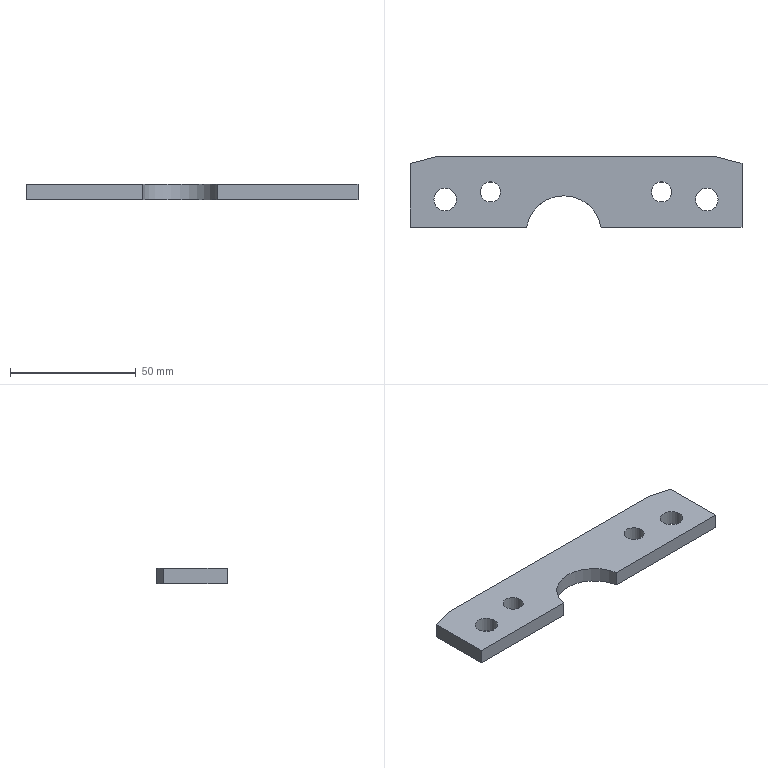Part | STEP file | gslz 2016.10.28-13_id730_x_t | 1 solid | 14 faces | box 132 x 28 x 6 mm | volume 18976 mm3 | plane 9 | cylinder 5 | commonest cylinder face diameters 8 x2 9 x2 30 x1
STEP:
#1=CARTESIAN_POINT('',(0.,0.,0.));
#2=DIRECTION('',(0.,0.,1.));
#3=DIRECTION('',(1.,0.,0.));
#4=AXIS2_PLACEMENT_3D('',#1,#2,#3);
#5=CARTESIAN_POINT('',(532.445,-295.75,0.));
#6=VERTEX_POINT('',#5);
#7=CARTESIAN_POINT('',(532.445,-295.75,6.));
#8=VERTEX_POINT('',#7);
#9=CARTESIAN_POINT('',(532.445,-295.75,290.));
#10=DIRECTION('',(0.,0.,1.));
#11=VECTOR('',#10,1.);
#12=LINE('',#9,#11);
#13=CARTESIAN_POINT('',(527.484,-295.75,16.));
#14=DIRECTION('',(0.,1.,0.));
#15=DIRECTION('',(0.,0.,-1.));
#16=AXIS2_PLACEMENT_3D('',#13,#14,#15);
#17=PLANE('',#16);
#18=CARTESIAN_POINT('',(-274.,-4.961));
#19=DIRECTION('',(-1.,0.));
#20=VECTOR('',#19,1.);
#21=LINE('',#18,#20);
#22=(GEOMETRIC_REPRESENTATION_CONTEXT(2)PARAMETRIC_REPRESENTATION_CONTEXT()REPRESENTATION_CONTEXT('',''));
#23=DEFINITIONAL_REPRESENTATION('',(#21),#22);
#24=PCURVE('',#17,#23);
#25=CARTESIAN_POINT('',(517.655,-298.25,290.));
#26=DIRECTION('',(0.,0.,-1.));
#27=DIRECTION('',(-1.,0.,0.));
#28=AXIS2_PLACEMENT_3D('',#25,#26,#27);
#29=CYLINDRICAL_SURFACE('',#28,15.);
#30=CARTESIAN_POINT('',(2.974,0.));
#31=DIRECTION('',(0.,-1.));
#32=VECTOR('',#31,1.);
#33=LINE('',#30,#32);
#34=(GEOMETRIC_REPRESENTATION_CONTEXT(2)PARAMETRIC_REPRESENTATION_CONTEXT()REPRESENTATION_CONTEXT('',''));
#35=DEFINITIONAL_REPRESENTATION('',(#33),#34);
#36=PCURVE('',#29,#35);
#37=SURFACE_CURVE('',#12,(#24,#36),.PCURVE_S1.);
#38=EDGE_CURVE('',#6,#8,#37,.T.);
#39=ORIENTED_EDGE('',*,*,#38,.F.);
#40=CARTESIAN_POINT('',(588.484,-295.75,0.));
#41=VERTEX_POINT('',#40);
#42=CARTESIAN_POINT('',(527.484,-295.75,0.));
#43=DIRECTION('',(-1.,0.,0.));
#44=VECTOR('',#43,1.);
#45=LINE('',#42,#44);
#46=CARTESIAN_POINT('',(16.,0.));
#47=DIRECTION('',(0.,1.));
#48=VECTOR('',#47,1.);
#49=LINE('',#46,#48);
#50=(GEOMETRIC_REPRESENTATION_CONTEXT(2)PARAMETRIC_REPRESENTATION_CONTEXT()REPRESENTATION_CONTEXT('',''));
#51=DEFINITIONAL_REPRESENTATION('',(#49),#50);
#52=PCURVE('',#17,#51);
#53=CARTESIAN_POINT('',(447.484,-295.75,0.));
#54=DIRECTION('',(0.,0.,1.));
#55=DIRECTION('',(1.,0.,0.));
#56=AXIS2_PLACEMENT_3D('',#53,#54,#55);
#57=PLANE('',#56);
#58=CARTESIAN_POINT('',(80.,0.));
#59=DIRECTION('',(-1.,0.));
#60=VECTOR('',#59,1.);
#61=LINE('',#58,#60);
#62=(GEOMETRIC_REPRESENTATION_CONTEXT(2)PARAMETRIC_REPRESENTATION_CONTEXT()REPRESENTATION_CONTEXT('',''));
#63=DEFINITIONAL_REPRESENTATION('',(#61),#62);
#64=PCURVE('',#57,#63);
#65=SURFACE_CURVE('',#45,(#52,#64),.PCURVE_S1.);
#66=EDGE_CURVE('',#41,#6,#65,.T.);
#67=ORIENTED_EDGE('',*,*,#66,.F.);
#68=CARTESIAN_POINT('',(588.484,-295.75,6.));
#69=VERTEX_POINT('',#68);
#70=CARTESIAN_POINT('',(588.484,-295.75,16.));
#71=DIRECTION('',(0.,0.,-1.));
#72=VECTOR('',#71,1.);
#73=LINE('',#70,#72);
#74=CARTESIAN_POINT('',(0.,-61.));
#75=DIRECTION('',(1.,0.));
#76=VECTOR('',#75,1.);
#77=LINE('',#74,#76);
#78=(GEOMETRIC_REPRESENTATION_CONTEXT(2)PARAMETRIC_REPRESENTATION_CONTEXT()REPRESENTATION_CONTEXT('',''));
#79=DEFINITIONAL_REPRESENTATION('',(#77),#78);
#80=PCURVE('',#17,#79);
#81=CARTESIAN_POINT('',(588.484,-262.75,16.));
#82=DIRECTION('',(-1.,0.,0.));
#83=DIRECTION('',(0.,0.,1.));
#84=AXIS2_PLACEMENT_3D('',#81,#82,#83);
#85=PLANE('',#84);
#86=CARTESIAN_POINT('',(0.,-33.));
#87=DIRECTION('',(-1.,0.));
#88=VECTOR('',#87,1.);
#89=LINE('',#86,#88);
#90=(GEOMETRIC_REPRESENTATION_CONTEXT(2)PARAMETRIC_REPRESENTATION_CONTEXT()REPRESENTATION_CONTEXT('',''));
#91=DEFINITIONAL_REPRESENTATION('',(#89),#90);
#92=PCURVE('',#85,#91);
#93=SURFACE_CURVE('',#73,(#80,#92),.PCURVE_S1.);
#94=EDGE_CURVE('',#69,#41,#93,.T.);
#95=ORIENTED_EDGE('',*,*,#94,.F.);
#96=CARTESIAN_POINT('',(527.484,-295.75,6.));
#97=DIRECTION('',(1.,0.,0.));
#98=VECTOR('',#97,1.);
#99=LINE('',#96,#98);
#100=CARTESIAN_POINT('',(10.,0.));
#101=DIRECTION('',(0.,-1.));
#102=VECTOR('',#101,1.);
#103=LINE('',#100,#102);
#104=(GEOMETRIC_REPRESENTATION_CONTEXT(2)PARAMETRIC_REPRESENTATION_CONTEXT()REPRESENTATION_CONTEXT('',''));
#105=DEFINITIONAL_REPRESENTATION('',(#103),#104);
#106=PCURVE('',#17,#105);
#107=CARTESIAN_POINT('',(487.484,-265.25,6.));
#108=DIRECTION('',(0.,0.,-1.));
#109=DIRECTION('',(-1.,0.,0.));
#110=AXIS2_PLACEMENT_3D('',#107,#108,#109);
#111=PLANE('',#110);
#112=CARTESIAN_POINT('',(-40.,-30.5));
#113=DIRECTION('',(-1.,0.));
#114=VECTOR('',#113,1.);
#115=LINE('',#112,#114);
#116=(GEOMETRIC_REPRESENTATION_CONTEXT(2)PARAMETRIC_REPRESENTATION_CONTEXT()REPRESENTATION_CONTEXT('',''));
#117=DEFINITIONAL_REPRESENTATION('',(#115),#116);
#118=PCURVE('',#111,#117);
#119=SURFACE_CURVE('',#99,(#106,#118),.PCURVE_S1.);
#120=EDGE_CURVE('',#8,#69,#119,.T.);
#121=ORIENTED_EDGE('',*,*,#120,.F.);
#122=EDGE_LOOP('',(#39,#67,#95,#121));
#123=FACE_BOUND('',#122,.T.);
#124=ADVANCED_FACE('',(#123),#17,.F.);
#125=CARTESIAN_POINT('',(502.865,-295.75,6.));
#126=VERTEX_POINT('',#125);
#127=CARTESIAN_POINT('',(502.865,-295.75,0.));
#128=VERTEX_POINT('',#127);
#129=CARTESIAN_POINT('',(502.865,-295.75,290.));
#130=DIRECTION('',(0.,0.,-1.));
#131=VECTOR('',#130,1.);
#132=LINE('',#129,#131);
#133=CARTESIAN_POINT('',(527.484,-295.75,16.));
#134=DIRECTION('',(0.,1.,0.));
#135=DIRECTION('',(0.,0.,-1.));
#136=AXIS2_PLACEMENT_3D('',#133,#134,#135);
#137=PLANE('',#136);
#138=CARTESIAN_POINT('',(-274.,24.62));
#139=DIRECTION('',(1.,0.));
#140=VECTOR('',#139,1.);
#141=LINE('',#138,#140);
#142=(GEOMETRIC_REPRESENTATION_CONTEXT(2)PARAMETRIC_REPRESENTATION_CONTEXT()REPRESENTATION_CONTEXT('',''));
#143=DEFINITIONAL_REPRESENTATION('',(#141),#142);
#144=PCURVE('',#137,#143);
#145=CARTESIAN_POINT('',(0.1674,0.));
#146=DIRECTION('',(0.,1.));
#147=VECTOR('',#146,1.);
#148=LINE('',#145,#147);
#149=(GEOMETRIC_REPRESENTATION_CONTEXT(2)PARAMETRIC_REPRESENTATION_CONTEXT()REPRESENTATION_CONTEXT('',''));
#150=DEFINITIONAL_REPRESENTATION('',(#148),#149);
#151=PCURVE('',#29,#150);
#152=SURFACE_CURVE('',#132,(#144,#151),.PCURVE_S1.);
#153=EDGE_CURVE('',#126,#128,#152,.T.);
#154=ORIENTED_EDGE('',*,*,#153,.F.);
#155=CARTESIAN_POINT('',(456.484,-295.75,6.));
#156=VERTEX_POINT('',#155);
#157=CARTESIAN_POINT('',(527.484,-295.75,6.));
#158=DIRECTION('',(1.,0.,0.));
#159=VECTOR('',#158,1.);
#160=LINE('',#157,#159);
#161=CARTESIAN_POINT('',(10.,0.));
#162=DIRECTION('',(0.,-1.));
#163=VECTOR('',#162,1.);
#164=LINE('',#161,#163);
#165=(GEOMETRIC_REPRESENTATION_CONTEXT(2)PARAMETRIC_REPRESENTATION_CONTEXT()REPRESENTATION_CONTEXT('',''));
#166=DEFINITIONAL_REPRESENTATION('',(#164),#165);
#167=PCURVE('',#137,#166);
#168=CARTESIAN_POINT('',(-40.,-30.5));
#169=DIRECTION('',(-1.,0.));
#170=VECTOR('',#169,1.);
#171=LINE('',#168,#170);
#172=(GEOMETRIC_REPRESENTATION_CONTEXT(2)PARAMETRIC_REPRESENTATION_CONTEXT()REPRESENTATION_CONTEXT('',''));
#173=DEFINITIONAL_REPRESENTATION('',(#171),#172);
#174=PCURVE('',#111,#173);
#175=SURFACE_CURVE('',#160,(#167,#174),.PCURVE_S1.);
#176=EDGE_CURVE('',#156,#126,#175,.T.);
#177=ORIENTED_EDGE('',*,*,#176,.F.);
#178=CARTESIAN_POINT('',(456.484,-295.75,0.));
#179=VERTEX_POINT('',#178);
#180=CARTESIAN_POINT('',(456.484,-295.75,16.));
#181=DIRECTION('',(0.,0.,-1.));
#182=VECTOR('',#181,1.);
#183=LINE('',#180,#182);
#184=CARTESIAN_POINT('',(0.,71.));
#185=DIRECTION('',(1.,0.));
#186=VECTOR('',#185,1.);
#187=LINE('',#184,#186);
#188=(GEOMETRIC_REPRESENTATION_CONTEXT(2)PARAMETRIC_REPRESENTATION_CONTEXT()REPRESENTATION_CONTEXT('',''));
#189=DEFINITIONAL_REPRESENTATION('',(#187),#188);
#190=PCURVE('',#137,#189);
#191=CARTESIAN_POINT('',(456.484,-295.75,16.));
#192=DIRECTION('',(1.,0.,0.));
#193=DIRECTION('',(0.,0.,-1.));
#194=AXIS2_PLACEMENT_3D('',#191,#192,#193);
#195=PLANE('',#194);
#196=CARTESIAN_POINT('',(0.,0.));
#197=DIRECTION('',(1.,0.));
#198=VECTOR('',#197,1.);
#199=LINE('',#196,#198);
#200=(GEOMETRIC_REPRESENTATION_CONTEXT(2)PARAMETRIC_REPRESENTATION_CONTEXT()REPRESENTATION_CONTEXT('',''));
#201=DEFINITIONAL_REPRESENTATION('',(#199),#200);
#202=PCURVE('',#195,#201);
#203=SURFACE_CURVE('',#183,(#190,#202),.PCURVE_S1.);
#204=EDGE_CURVE('',#156,#179,#203,.T.);
#205=ORIENTED_EDGE('',*,*,#204,.T.);
#206=CARTESIAN_POINT('',(527.484,-295.75,0.));
#207=DIRECTION('',(-1.,0.,0.));
#208=VECTOR('',#207,1.);
#209=LINE('',#206,#208);
#210=CARTESIAN_POINT('',(16.,0.));
#211=DIRECTION('',(0.,1.));
#212=VECTOR('',#211,1.);
#213=LINE('',#210,#212);
#214=(GEOMETRIC_REPRESENTATION_CONTEXT(2)PARAMETRIC_REPRESENTATION_CONTEXT()REPRESENTATION_CONTEXT('',''));
#215=DEFINITIONAL_REPRESENTATION('',(#213),#214);
#216=PCURVE('',#137,#215);
#217=CARTESIAN_POINT('',(80.,0.));
#218=DIRECTION('',(-1.,0.));
#219=VECTOR('',#218,1.);
#220=LINE('',#217,#219);
#221=(GEOMETRIC_REPRESENTATION_CONTEXT(2)PARAMETRIC_REPRESENTATION_CONTEXT()REPRESENTATION_CONTEXT('',''));
#222=DEFINITIONAL_REPRESENTATION('',(#220),#221);
#223=PCURVE('',#57,#222);
#224=SURFACE_CURVE('',#209,(#216,#223),.PCURVE_S1.);
#225=EDGE_CURVE('',#128,#179,#224,.T.);
#226=ORIENTED_EDGE('',*,*,#225,.F.);
#227=EDGE_LOOP('',(#154,#177,#205,#226));
#228=FACE_BOUND('',#227,.T.);
#229=ADVANCED_FACE('',(#228),#137,.F.);
#230=CARTESIAN_POINT('',(569.984,-284.75,6.));
#231=VERTEX_POINT('',#230);
#232=CARTESIAN_POINT('',(574.484,-284.75,6.));
#233=DIRECTION('',(0.,0.,-1.));
#234=DIRECTION('',(-1.,0.,0.));
#235=AXIS2_PLACEMENT_3D('',#232,#233,#234);
#236=CIRCLE('',#235,4.5);
#237=CARTESIAN_POINT('',(-87.,-19.5));
#238=DIRECTION('',(1.,0.));
#239=AXIS2_PLACEMENT_2D('',#237,#238);
#240=CIRCLE('',#239,4.5);
#241=(GEOMETRIC_REPRESENTATION_CONTEXT(2)PARAMETRIC_REPRESENTATION_CONTEXT()REPRESENTATION_CONTEXT('',''));
#242=DEFINITIONAL_REPRESENTATION('',(#240),#241);
#243=PCURVE('',#111,#242);
#244=CARTESIAN_POINT('',(574.484,-284.75,47.));
#245=DIRECTION('',(0.,0.,-1.));
#246=DIRECTION('',(-1.,0.,0.));
#247=AXIS2_PLACEMENT_3D('',#244,#245,#246);
#248=CYLINDRICAL_SURFACE('',#247,4.5);
#249=CARTESIAN_POINT('',(0.,41.));
#250=DIRECTION('',(1.,0.));
#251=VECTOR('',#250,1.);
#252=LINE('',#249,#251);
#253=(GEOMETRIC_REPRESENTATION_CONTEXT(2)PARAMETRIC_REPRESENTATION_CONTEXT()REPRESENTATION_CONTEXT('',''));
#254=DEFINITIONAL_REPRESENTATION('',(#252),#253);
#255=PCURVE('',#248,#254);
#256=SURFACE_CURVE('',#236,(#243,#255),.PCURVE_S1.);
#257=EDGE_CURVE('',#231,#231,#256,.T.);
#258=ORIENTED_EDGE('',*,*,#257,.T.);
#259=EDGE_LOOP('',(#258));
#260=FACE_BOUND('',#259,.T.);
#261=CARTESIAN_POINT('',(484.484,-281.75,6.));
#262=VERTEX_POINT('',#261);
#263=CARTESIAN_POINT('',(492.484,-281.75,6.));
#264=VERTEX_POINT('',#263);
#265=CARTESIAN_POINT('',(488.484,-281.75,6.));
#266=DIRECTION('',(0.,0.,-1.));
#267=DIRECTION('',(-1.,0.,0.));
#268=AXIS2_PLACEMENT_3D('',#265,#266,#267);
#269=CIRCLE('',#268,4.);
#270=CARTESIAN_POINT('',(-1.,-16.5));
#271=DIRECTION('',(1.,0.));
#272=AXIS2_PLACEMENT_2D('',#270,#271);
#273=CIRCLE('',#272,4.);
#274=(GEOMETRIC_REPRESENTATION_CONTEXT(2)PARAMETRIC_REPRESENTATION_CONTEXT()REPRESENTATION_CONTEXT('',''));
#275=DEFINITIONAL_REPRESENTATION('',(#273),#274);
#276=PCURVE('',#111,#275);
#277=CARTESIAN_POINT('',(488.484,-281.75,-73.));
#278=DIRECTION('',(0.,0.,1.));
#279=DIRECTION('',(1.,0.,0.));
#280=AXIS2_PLACEMENT_3D('',#277,#278,#279);
#281=CYLINDRICAL_SURFACE('',#280,4.);
#282=CARTESIAN_POINT('',(3.142,79.));
#283=DIRECTION('',(-1.,0.));
#284=VECTOR('',#283,1.);
#285=LINE('',#282,#284);
#286=(GEOMETRIC_REPRESENTATION_CONTEXT(2)PARAMETRIC_REPRESENTATION_CONTEXT()REPRESENTATION_CONTEXT('',''));
#287=DEFINITIONAL_REPRESENTATION('',(#285),#286);
#288=PCURVE('',#281,#287);
#289=SURFACE_CURVE('',#269,(#276,#288),.PCURVE_S1.);
#290=EDGE_CURVE('',#262,#264,#289,.T.);
#291=ORIENTED_EDGE('',*,*,#290,.T.);
#292=CARTESIAN_POINT('',(488.484,-281.75,6.));
#293=DIRECTION('',(0.,0.,-1.));
#294=DIRECTION('',(-1.,0.,0.));
#295=AXIS2_PLACEMENT_3D('',#292,#293,#294);
#296=CIRCLE('',#295,4.);
#297=CARTESIAN_POINT('',(-1.,-16.5));
#298=DIRECTION('',(1.,0.));
#299=AXIS2_PLACEMENT_2D('',#297,#298);
#300=CIRCLE('',#299,4.);
#301=(GEOMETRIC_REPRESENTATION_CONTEXT(2)PARAMETRIC_REPRESENTATION_CONTEXT()REPRESENTATION_CONTEXT('',''));
#302=DEFINITIONAL_REPRESENTATION('',(#300),#301);
#303=PCURVE('',#111,#302);
#304=CARTESIAN_POINT('',(9.425,79.));
#305=DIRECTION('',(-1.,0.));
#306=VECTOR('',#305,1.);
#307=LINE('',#304,#306);
#308=(GEOMETRIC_REPRESENTATION_CONTEXT(2)PARAMETRIC_REPRESENTATION_CONTEXT()REPRESENTATION_CONTEXT('',''));
#309=DEFINITIONAL_REPRESENTATION('',(#307),#308);
#310=PCURVE('',#281,#309);
#311=SURFACE_CURVE('',#296,(#303,#310),.PCURVE_S1.);
#312=EDGE_CURVE('',#264,#262,#311,.T.);
#313=ORIENTED_EDGE('',*,*,#312,.T.);
#314=EDGE_LOOP('',(#291,#313));
#315=FACE_BOUND('',#314,.T.);
#316=CARTESIAN_POINT('',(552.484,-281.75,6.));
#317=VERTEX_POINT('',#316);
#318=CARTESIAN_POINT('',(560.484,-281.75,6.));
#319=VERTEX_POINT('',#318);
#320=CARTESIAN_POINT('',(556.484,-281.75,6.));
#321=DIRECTION('',(0.,0.,1.));
#322=DIRECTION('',(-1.,0.,0.));
#323=AXIS2_PLACEMENT_3D('',#320,#321,#322);
#324=CIRCLE('',#323,4.);
#325=CARTESIAN_POINT('',(-65.,-16.5));
#326=CARTESIAN_POINT('',(-65.,-23.428));
#327=CARTESIAN_POINT('',(-71.,-19.964));
#328=CARTESIAN_POINT('',(-77.,-16.5));
#329=CARTESIAN_POINT('',(-71.,-13.036));
#330=CARTESIAN_POINT('',(-65.,-9.572));
#331=CARTESIAN_POINT('',(-65.,-16.5));
#332=(BOUNDED_CURVE()B_SPLINE_CURVE(2,(#325,#326,#327,#328,#329,#330,#331),.UNSPECIFIED.,.T.,.F.)B_SPLINE_CURVE_WITH_KNOTS((1,2,2,2,2,1),(-2.094,0.,2.094,4.189,6.283,8.378),.UNSPECIFIED.)CURVE()GEOMETRIC_REPRESENTATION_ITEM()RATIONAL_B_SPLINE_CURVE((1.,0.5,1.,0.5,1.,0.5,1.))REPRESENTATION_ITEM(''));
#333=(GEOMETRIC_REPRESENTATION_CONTEXT(2)PARAMETRIC_REPRESENTATION_CONTEXT()REPRESENTATION_CONTEXT('',''));
#334=DEFINITIONAL_REPRESENTATION('',(#332),#333);
#335=PCURVE('',#111,#334);
#336=CARTESIAN_POINT('',(556.484,-281.75,-73.));
#337=DIRECTION('',(0.,0.,1.));
#338=DIRECTION('',(1.,0.,0.));
#339=AXIS2_PLACEMENT_3D('',#336,#337,#338);
#340=CYLINDRICAL_SURFACE('',#339,4.);
#341=CARTESIAN_POINT('',(3.142,79.));
#342=DIRECTION('',(1.,0.));
#343=VECTOR('',#342,1.);
#344=LINE('',#341,#343);
#345=(GEOMETRIC_REPRESENTATION_CONTEXT(2)PARAMETRIC_REPRESENTATION_CONTEXT()REPRESENTATION_CONTEXT('',''));
#346=DEFINITIONAL_REPRESENTATION('',(#344),#345);
#347=PCURVE('',#340,#346);
#348=SURFACE_CURVE('',#324,(#335,#347),.PCURVE_S1.);
#349=EDGE_CURVE('',#317,#319,#348,.T.);
#350=ORIENTED_EDGE('',*,*,#349,.F.);
#351=CARTESIAN_POINT('',(556.484,-281.75,6.));
#352=DIRECTION('',(0.,0.,1.));
#353=DIRECTION('',(-1.,0.,0.));
#354=AXIS2_PLACEMENT_3D('',#351,#352,#353);
#355=CIRCLE('',#354,4.);
#356=CARTESIAN_POINT('',(-65.,-16.5));
#357=CARTESIAN_POINT('',(-65.,-23.428));
#358=CARTESIAN_POINT('',(-71.,-19.964));
#359=CARTESIAN_POINT('',(-77.,-16.5));
#360=CARTESIAN_POINT('',(-71.,-13.036));
#361=CARTESIAN_POINT('',(-65.,-9.572));
#362=CARTESIAN_POINT('',(-65.,-16.5));
#363=(BOUNDED_CURVE()B_SPLINE_CURVE(2,(#356,#357,#358,#359,#360,#361,#362),.UNSPECIFIED.,.T.,.F.)B_SPLINE_CURVE_WITH_KNOTS((1,2,2,2,2,1),(-2.094,0.,2.094,4.189,6.283,8.378),.UNSPECIFIED.)CURVE()GEOMETRIC_REPRESENTATION_ITEM()RATIONAL_B_SPLINE_CURVE((1.,0.5,1.,0.5,1.,0.5,1.))REPRESENTATION_ITEM(''));
#364=(GEOMETRIC_REPRESENTATION_CONTEXT(2)PARAMETRIC_REPRESENTATION_CONTEXT()REPRESENTATION_CONTEXT('',''));
#365=DEFINITIONAL_REPRESENTATION('',(#363),#364);
#366=PCURVE('',#111,#365);
#367=CARTESIAN_POINT('',(-3.142,79.));
#368=DIRECTION('',(1.,0.));
#369=VECTOR('',#368,1.);
#370=LINE('',#367,#369);
#371=(GEOMETRIC_REPRESENTATION_CONTEXT(2)PARAMETRIC_REPRESENTATION_CONTEXT()REPRESENTATION_CONTEXT('',''));
#372=DEFINITIONAL_REPRESENTATION('',(#370),#371);
#373=PCURVE('',#340,#372);
#374=SURFACE_CURVE('',#355,(#366,#373),.PCURVE_S1.);
#375=EDGE_CURVE('',#319,#317,#374,.T.);
#376=ORIENTED_EDGE('',*,*,#375,.F.);
#377=EDGE_LOOP('',(#350,#376));
#378=FACE_BOUND('',#377,.T.);
#379=CARTESIAN_POINT('',(465.984,-284.75,6.));
#380=VERTEX_POINT('',#379);
#381=CARTESIAN_POINT('',(470.484,-284.75,6.));
#382=DIRECTION('',(0.,0.,1.));
#383=DIRECTION('',(-1.,0.,0.));
#384=AXIS2_PLACEMENT_3D('',#381,#382,#383);
#385=CIRCLE('',#384,4.5);
#386=CARTESIAN_POINT('',(21.5,-19.5));
#387=CARTESIAN_POINT('',(21.5,-27.294));
#388=CARTESIAN_POINT('',(14.75,-23.397));
#389=CARTESIAN_POINT('',(8.,-19.5));
#390=CARTESIAN_POINT('',(14.75,-15.603));
#391=CARTESIAN_POINT('',(21.5,-11.706));
#392=CARTESIAN_POINT('',(21.5,-19.5));
#393=(BOUNDED_CURVE()B_SPLINE_CURVE(2,(#386,#387,#388,#389,#390,#391,#392),.UNSPECIFIED.,.T.,.F.)B_SPLINE_CURVE_WITH_KNOTS((1,2,2,2,2,1),(-2.094,0.,2.094,4.189,6.283,8.378),.UNSPECIFIED.)CURVE()GEOMETRIC_REPRESENTATION_ITEM()RATIONAL_B_SPLINE_CURVE((1.,0.5,1.,0.5,1.,0.5,1.))REPRESENTATION_ITEM(''));
#394=(GEOMETRIC_REPRESENTATION_CONTEXT(2)PARAMETRIC_REPRESENTATION_CONTEXT()REPRESENTATION_CONTEXT('',''));
#395=DEFINITIONAL_REPRESENTATION('',(#393),#394);
#396=PCURVE('',#111,#395);
#397=CARTESIAN_POINT('',(470.484,-284.75,47.));
#398=DIRECTION('',(0.,0.,-1.));
#399=DIRECTION('',(-1.,0.,0.));
#400=AXIS2_PLACEMENT_3D('',#397,#398,#399);
#401=CYLINDRICAL_SURFACE('',#400,4.5);
#402=CARTESIAN_POINT('',(6.283,41.));
#403=DIRECTION('',(-1.,0.));
#404=VECTOR('',#403,1.);
#405=LINE('',#402,#404);
#406=(GEOMETRIC_REPRESENTATION_CONTEXT(2)PARAMETRIC_REPRESENTATION_CONTEXT()REPRESENTATION_CONTEXT('',''));
#407=DEFINITIONAL_REPRESENTATION('',(#405),#406);
#408=PCURVE('',#401,#407);
#409=SURFACE_CURVE('',#385,(#396,#408),.PCURVE_S1.);
#410=EDGE_CURVE('',#380,#380,#409,.T.);
#411=ORIENTED_EDGE('',*,*,#410,.F.);
#412=EDGE_LOOP('',(#411));
#413=FACE_BOUND('',#412,.T.);
#414=CARTESIAN_POINT('',(517.655,-298.25,6.));
#415=DIRECTION('',(0.,0.,1.));
#416=DIRECTION('',(-1.,0.,0.));
#417=AXIS2_PLACEMENT_3D('',#414,#415,#416);
#418=CIRCLE('',#417,15.);
#419=CARTESIAN_POINT('',(-15.17,-33.));
#420=CARTESIAN_POINT('',(-15.17,-58.981));
#421=CARTESIAN_POINT('',(-37.67,-45.99));
#422=CARTESIAN_POINT('',(-60.17,-33.));
#423=CARTESIAN_POINT('',(-37.67,-20.009));
#424=CARTESIAN_POINT('',(-15.17,-7.019));
#425=CARTESIAN_POINT('',(-15.17,-33.));
#426=(BOUNDED_CURVE()B_SPLINE_CURVE(2,(#419,#420,#421,#422,#423,#424,#425),.UNSPECIFIED.,.T.,.F.)B_SPLINE_CURVE_WITH_KNOTS((1,2,2,2,2,1),(-2.094,0.,2.094,4.189,6.283,8.378),.UNSPECIFIED.)CURVE()GEOMETRIC_REPRESENTATION_ITEM()RATIONAL_B_SPLINE_CURVE((1.,0.5,1.,0.5,1.,0.5,1.))REPRESENTATION_ITEM(''));
#427=(GEOMETRIC_REPRESENTATION_CONTEXT(2)PARAMETRIC_REPRESENTATION_CONTEXT()REPRESENTATION_CONTEXT('',''));
#428=DEFINITIONAL_REPRESENTATION('',(#426),#427);
#429=PCURVE('',#111,#428);
#430=CARTESIAN_POINT('',(6.283,284.));
#431=DIRECTION('',(-1.,0.));
#432=VECTOR('',#431,1.);
#433=LINE('',#430,#432);
#434=(GEOMETRIC_REPRESENTATION_CONTEXT(2)PARAMETRIC_REPRESENTATION_CONTEXT()REPRESENTATION_CONTEXT('',''));
#435=DEFINITIONAL_REPRESENTATION('',(#433),#434);
#436=PCURVE('',#29,#435);
#437=SURFACE_CURVE('',#418,(#429,#436),.PCURVE_S1.);
#438=EDGE_CURVE('',#8,#126,#437,.T.);
#439=ORIENTED_EDGE('',*,*,#438,.F.);
#440=ORIENTED_EDGE('',*,*,#120,.T.);
#441=CARTESIAN_POINT('',(588.484,-270.429,6.));
#442=VERTEX_POINT('',#441);
#443=CARTESIAN_POINT('',(588.484,-262.75,6.));
#444=DIRECTION('',(0.,1.,0.));
#445=VECTOR('',#444,1.);
#446=LINE('',#443,#445);
#447=CARTESIAN_POINT('',(-101.,2.5));
#448=DIRECTION('',(0.,1.));
#449=VECTOR('',#448,1.);
#450=LINE('',#447,#449);
#451=(GEOMETRIC_REPRESENTATION_CONTEXT(2)PARAMETRIC_REPRESENTATION_CONTEXT()REPRESENTATION_CONTEXT('',''));
#452=DEFINITIONAL_REPRESENTATION('',(#450),#451);
#453=PCURVE('',#111,#452);
#454=CARTESIAN_POINT('',(-10.,0.));
#455=DIRECTION('',(0.,1.));
#456=VECTOR('',#455,1.);
#457=LINE('',#454,#456);
#458=(GEOMETRIC_REPRESENTATION_CONTEXT(2)PARAMETRIC_REPRESENTATION_CONTEXT()REPRESENTATION_CONTEXT('',''));
#459=DEFINITIONAL_REPRESENTATION('',(#457),#458);
#460=PCURVE('',#85,#459);
#461=SURFACE_CURVE('',#446,(#453,#460),.PCURVE_S1.);
#462=EDGE_CURVE('',#69,#442,#461,.T.);
#463=ORIENTED_EDGE('',*,*,#462,.T.);
#464=CARTESIAN_POINT('',(578.485,-267.75,6.));
#465=VERTEX_POINT('',#464);
#466=CARTESIAN_POINT('',(578.485,-267.75,6.));
#467=DIRECTION('',(-0.9659,0.2588,0.));
#468=VECTOR('',#467,1.);
#469=LINE('',#466,#468);
#470=CARTESIAN_POINT('',(-91.001,-2.5));
#471=DIRECTION('',(0.9659,0.2588));
#472=VECTOR('',#471,1.);
#473=LINE('',#470,#472);
#474=(GEOMETRIC_REPRESENTATION_CONTEXT(2)PARAMETRIC_REPRESENTATION_CONTEXT()REPRESENTATION_CONTEXT('',''));
#475=DEFINITIONAL_REPRESENTATION('',(#473),#474);
#476=PCURVE('',#111,#475);
#477=CARTESIAN_POINT('',(578.485,-267.75,8.));
#478=DIRECTION('',(-0.2588,-0.9659,0.));
#479=DIRECTION('',(-0.9659,0.2588,0.));
#480=AXIS2_PLACEMENT_3D('',#477,#478,#479);
#481=PLANE('',#480);
#482=CARTESIAN_POINT('',(0.,2.));
#483=DIRECTION('',(1.,0.));
#484=VECTOR('',#483,1.);
#485=LINE('',#482,#484);
#486=(GEOMETRIC_REPRESENTATION_CONTEXT(2)PARAMETRIC_REPRESENTATION_CONTEXT()REPRESENTATION_CONTEXT('',''));
#487=DEFINITIONAL_REPRESENTATION('',(#485),#486);
#488=PCURVE('',#481,#487);
#489=SURFACE_CURVE('',#469,(#476,#488),.PCURVE_S1.);
#490=EDGE_CURVE('',#442,#465,#489,.T.);
#491=ORIENTED_EDGE('',*,*,#490,.T.);
#492=CARTESIAN_POINT('',(466.486,-267.75,6.));
#493=VERTEX_POINT('',#492);
#494=CARTESIAN_POINT('',(457.486,-267.75,6.));
#495=DIRECTION('',(-1.,0.,0.));
#496=VECTOR('',#495,1.);
#497=LINE('',#494,#496);
#498=CARTESIAN_POINT('',(29.998,-2.5));
#499=DIRECTION('',(1.,0.));
#500=VECTOR('',#499,1.);
#501=LINE('',#498,#500);
#502=(GEOMETRIC_REPRESENTATION_CONTEXT(2)PARAMETRIC_REPRESENTATION_CONTEXT()REPRESENTATION_CONTEXT('',''));
#503=DEFINITIONAL_REPRESENTATION('',(#501),#502);
#504=PCURVE('',#111,#503);
#505=CARTESIAN_POINT('',(457.486,-267.75,8.));
#506=DIRECTION('',(0.,-1.,0.));
#507=DIRECTION('',(0.,0.,1.));
#508=AXIS2_PLACEMENT_3D('',#505,#506,#507);
#509=PLANE('',#508);
#510=CARTESIAN_POINT('',(-2.,0.));
#511=DIRECTION('',(0.,1.));
#512=VECTOR('',#511,1.);
#513=LINE('',#510,#512);
#514=(GEOMETRIC_REPRESENTATION_CONTEXT(2)PARAMETRIC_REPRESENTATION_CONTEXT()REPRESENTATION_CONTEXT('',''));
#515=DEFINITIONAL_REPRESENTATION('',(#513),#514);
#516=PCURVE('',#509,#515);
#517=SURFACE_CURVE('',#497,(#504,#516),.PCURVE_S1.);
#518=EDGE_CURVE('',#465,#493,#517,.T.);
#519=ORIENTED_EDGE('',*,*,#518,.T.);
#520=CARTESIAN_POINT('',(456.484,-270.43,6.));
#521=VERTEX_POINT('',#520);
#522=CARTESIAN_POINT('',(456.484,-270.43,6.));
#523=DIRECTION('',(-0.9659,-0.2588,0.));
#524=VECTOR('',#523,1.);
#525=LINE('',#522,#524);
#526=CARTESIAN_POINT('',(31.,-5.18));
#527=DIRECTION('',(0.9659,-0.2588));
#528=VECTOR('',#527,1.);
#529=LINE('',#526,#528);
#530=(GEOMETRIC_REPRESENTATION_CONTEXT(2)PARAMETRIC_REPRESENTATION_CONTEXT()REPRESENTATION_CONTEXT('',''));
#531=DEFINITIONAL_REPRESENTATION('',(#529),#530);
#532=PCURVE('',#111,#531);
#533=CARTESIAN_POINT('',(456.484,-270.43,8.));
#534=DIRECTION('',(0.2588,-0.9659,0.));
#535=DIRECTION('',(-0.9659,-0.2588,0.));
#536=AXIS2_PLACEMENT_3D('',#533,#534,#535);
#537=PLANE('',#536);
#538=CARTESIAN_POINT('',(0.,2.));
#539=DIRECTION('',(1.,0.));
#540=VECTOR('',#539,1.);
#541=LINE('',#538,#540);
#542=(GEOMETRIC_REPRESENTATION_CONTEXT(2)PARAMETRIC_REPRESENTATION_CONTEXT()REPRESENTATION_CONTEXT('',''));
#543=DEFINITIONAL_REPRESENTATION('',(#541),#542);
#544=PCURVE('',#537,#543);
#545=SURFACE_CURVE('',#525,(#532,#544),.PCURVE_S1.);
#546=EDGE_CURVE('',#493,#521,#545,.T.);
#547=ORIENTED_EDGE('',*,*,#546,.T.);
#548=CARTESIAN_POINT('',(456.484,-295.75,6.));
#549=DIRECTION('',(0.,-1.,0.));
#550=VECTOR('',#549,1.);
#551=LINE('',#548,#550);
#552=CARTESIAN_POINT('',(31.,-30.5));
#553=DIRECTION('',(0.,-1.));
#554=VECTOR('',#553,1.);
#555=LINE('',#552,#554);
#556=(GEOMETRIC_REPRESENTATION_CONTEXT(2)PARAMETRIC_REPRESENTATION_CONTEXT()REPRESENTATION_CONTEXT('',''));
#557=DEFINITIONAL_REPRESENTATION('',(#555),#556);
#558=PCURVE('',#111,#557);
#559=CARTESIAN_POINT('',(10.,0.));
#560=DIRECTION('',(0.,-1.));
#561=VECTOR('',#560,1.);
#562=LINE('',#559,#561);
#563=(GEOMETRIC_REPRESENTATION_CONTEXT(2)PARAMETRIC_REPRESENTATION_CONTEXT()REPRESENTATION_CONTEXT('',''));
#564=DEFINITIONAL_REPRESENTATION('',(#562),#563);
#565=PCURVE('',#195,#564);
#566=SURFACE_CURVE('',#551,(#558,#565),.PCURVE_S1.);
#567=EDGE_CURVE('',#521,#156,#566,.T.);
#568=ORIENTED_EDGE('',*,*,#567,.T.);
#569=ORIENTED_EDGE('',*,*,#176,.T.);
#570=EDGE_LOOP('',(#439,#440,#463,#491,#519,#547,#568,#569));
#571=FACE_BOUND('',#570,.T.);
#572=ADVANCED_FACE('',(#260,#315,#378,#413,#571),#111,.F.);
#573=ORIENTED_EDGE('',*,*,#290,.T.);
#574=CARTESIAN_POINT('',(492.484,-281.75,0.));
#575=VERTEX_POINT('',#574);
#576=CARTESIAN_POINT('',(492.484,-281.75,0.));
#577=CARTESIAN_POINT('',(492.484,-281.75,6.));
#578=B_SPLINE_CURVE_WITH_KNOTS('',1,(#576,#577),.UNSPECIFIED.,.F.,.F.,(2,2),(73.,79.),.PIECEWISE_BEZIER_KNOTS.);
#579=CARTESIAN_POINT('',(0.,0.));
#580=DIRECTION('',(0.,1.));
#581=VECTOR('',#580,1.);
#582=LINE('',#579,#581);
#583=(GEOMETRIC_REPRESENTATION_CONTEXT(2)PARAMETRIC_REPRESENTATION_CONTEXT()REPRESENTATION_CONTEXT('',''));
#584=DEFINITIONAL_REPRESENTATION('',(#582),#583);
#585=PCURVE('',#281,#584);
#586=CARTESIAN_POINT('',(6.283,0.));
#587=DIRECTION('',(0.,1.));
#588=VECTOR('',#587,1.);
#589=LINE('',#586,#588);
#590=(GEOMETRIC_REPRESENTATION_CONTEXT(2)PARAMETRIC_REPRESENTATION_CONTEXT()REPRESENTATION_CONTEXT('',''));
#591=DEFINITIONAL_REPRESENTATION('',(#589),#590);
#592=PCURVE('',#281,#591);
#593=SEAM_CURVE('',#578,(#585,#592),.PCURVE_S1.);
#594=EDGE_CURVE('',#575,#264,#593,.T.);
#595=ORIENTED_EDGE('',*,*,#594,.F.);
#596=CARTESIAN_POINT('',(488.484,-281.75,0.));
#597=DIRECTION('',(0.,0.,1.));
#598=DIRECTION('',(1.,0.,0.));
#599=AXIS2_PLACEMENT_3D('',#596,#597,#598);
#600=CIRCLE('',#599,4.);
#601=CARTESIAN_POINT('',(0.,73.));
#602=DIRECTION('',(1.,0.));
#603=VECTOR('',#602,1.);
#604=LINE('',#601,#603);
#605=(GEOMETRIC_REPRESENTATION_CONTEXT(2)PARAMETRIC_REPRESENTATION_CONTEXT()REPRESENTATION_CONTEXT('',''));
#606=DEFINITIONAL_REPRESENTATION('',(#604),#605);
#607=PCURVE('',#281,#606);
#608=CARTESIAN_POINT('',(41.,14.));
#609=DIRECTION('',(1.,0.));
#610=AXIS2_PLACEMENT_2D('',#608,#609);
#611=CIRCLE('',#610,4.);
#612=(GEOMETRIC_REPRESENTATION_CONTEXT(2)PARAMETRIC_REPRESENTATION_CONTEXT()REPRESENTATION_CONTEXT('',''));
#613=DEFINITIONAL_REPRESENTATION('',(#611),#612);
#614=PCURVE('',#57,#613);
#615=SURFACE_CURVE('',#600,(#607,#614),.PCURVE_S1.);
#616=EDGE_CURVE('',#575,#575,#615,.T.);
#617=ORIENTED_EDGE('',*,*,#616,.T.);
#618=ORIENTED_EDGE('',*,*,#594,.T.);
#619=ORIENTED_EDGE('',*,*,#312,.T.);
#620=EDGE_LOOP('',(#573,#595,#617,#618,#619));
#621=FACE_BOUND('',#620,.F.);
#622=ADVANCED_FACE('',(#621),#281,.F.);
#623=ORIENTED_EDGE('',*,*,#375,.F.);
#624=CARTESIAN_POINT('',(560.484,-281.75,0.));
#625=VERTEX_POINT('',#624);
#626=CARTESIAN_POINT('',(560.484,-281.75,0.));
#627=CARTESIAN_POINT('',(560.484,-281.75,6.));
#628=B_SPLINE_CURVE_WITH_KNOTS('',1,(#626,#627),.UNSPECIFIED.,.F.,.F.,(2,2),(73.,79.),.PIECEWISE_BEZIER_KNOTS.);
#629=CARTESIAN_POINT('',(0.,0.));
#630=DIRECTION('',(0.,1.));
#631=VECTOR('',#630,1.);
#632=LINE('',#629,#631);
#633=(GEOMETRIC_REPRESENTATION_CONTEXT(2)PARAMETRIC_REPRESENTATION_CONTEXT()REPRESENTATION_CONTEXT('',''));
#634=DEFINITIONAL_REPRESENTATION('',(#632),#633);
#635=PCURVE('',#340,#634);
#636=CARTESIAN_POINT('',(6.283,0.));
#637=DIRECTION('',(0.,1.));
#638=VECTOR('',#637,1.);
#639=LINE('',#636,#638);
#640=(GEOMETRIC_REPRESENTATION_CONTEXT(2)PARAMETRIC_REPRESENTATION_CONTEXT()REPRESENTATION_CONTEXT('',''));
#641=DEFINITIONAL_REPRESENTATION('',(#639),#640);
#642=PCURVE('',#340,#641);
#643=SEAM_CURVE('',#628,(#635,#642),.PCURVE_S1.);
#644=EDGE_CURVE('',#625,#319,#643,.T.);
#645=ORIENTED_EDGE('',*,*,#644,.F.);
#646=CARTESIAN_POINT('',(556.484,-281.75,0.));
#647=DIRECTION('',(0.,0.,-1.));
#648=DIRECTION('',(1.,0.,0.));
#649=AXIS2_PLACEMENT_3D('',#646,#647,#648);
#650=CIRCLE('',#649,4.);
#651=CARTESIAN_POINT('',(6.283,73.));
#652=DIRECTION('',(-1.,0.));
#653=VECTOR('',#652,1.);
#654=LINE('',#651,#653);
#655=(GEOMETRIC_REPRESENTATION_CONTEXT(2)PARAMETRIC_REPRESENTATION_CONTEXT()REPRESENTATION_CONTEXT('',''));
#656=DEFINITIONAL_REPRESENTATION('',(#654),#655);
#657=PCURVE('',#340,#656);
#658=CARTESIAN_POINT('',(113.,14.));
#659=CARTESIAN_POINT('',(113.,7.072));
#660=CARTESIAN_POINT('',(107.,10.536));
#661=CARTESIAN_POINT('',(101.,14.));
#662=CARTESIAN_POINT('',(107.,17.464));
#663=CARTESIAN_POINT('',(113.,20.928));
#664=CARTESIAN_POINT('',(113.,14.));
#665=(BOUNDED_CURVE()B_SPLINE_CURVE(2,(#658,#659,#660,#661,#662,#663,#664),.UNSPECIFIED.,.T.,.F.)B_SPLINE_CURVE_WITH_KNOTS((1,2,2,2,2,1),(-2.094,0.,2.094,4.189,6.283,8.378),.UNSPECIFIED.)CURVE()GEOMETRIC_REPRESENTATION_ITEM()RATIONAL_B_SPLINE_CURVE((1.,0.5,1.,0.5,1.,0.5,1.))REPRESENTATION_ITEM(''));
#666=(GEOMETRIC_REPRESENTATION_CONTEXT(2)PARAMETRIC_REPRESENTATION_CONTEXT()REPRESENTATION_CONTEXT('',''));
#667=DEFINITIONAL_REPRESENTATION('',(#665),#666);
#668=PCURVE('',#57,#667);
#669=SURFACE_CURVE('',#650,(#657,#668),.PCURVE_S1.);
#670=EDGE_CURVE('',#625,#625,#669,.T.);
#671=ORIENTED_EDGE('',*,*,#670,.F.);
#672=ORIENTED_EDGE('',*,*,#644,.T.);
#673=ORIENTED_EDGE('',*,*,#349,.F.);
#674=EDGE_LOOP('',(#623,#645,#671,#672,#673));
#675=FACE_BOUND('',#674,.F.);
#676=ADVANCED_FACE('',(#675),#340,.F.);
#677=ORIENTED_EDGE('',*,*,#410,.F.);
#678=CARTESIAN_POINT('',(465.984,-284.75,0.));
#679=VERTEX_POINT('',#678);
#680=CARTESIAN_POINT('',(465.984,-284.75,6.));
#681=CARTESIAN_POINT('',(465.984,-284.75,0.));
#682=B_SPLINE_CURVE_WITH_KNOTS('',1,(#680,#681),.UNSPECIFIED.,.F.,.F.,(2,2),(41.,47.),.PIECEWISE_BEZIER_KNOTS.);
#683=CARTESIAN_POINT('',(6.283,0.));
#684=DIRECTION('',(0.,1.));
#685=VECTOR('',#684,1.);
#686=LINE('',#683,#685);
#687=(GEOMETRIC_REPRESENTATION_CONTEXT(2)PARAMETRIC_REPRESENTATION_CONTEXT()REPRESENTATION_CONTEXT('',''));
#688=DEFINITIONAL_REPRESENTATION('',(#686),#687);
#689=PCURVE('',#401,#688);
#690=CARTESIAN_POINT('',(0.,0.));
#691=DIRECTION('',(0.,1.));
#692=VECTOR('',#691,1.);
#693=LINE('',#690,#692);
#694=(GEOMETRIC_REPRESENTATION_CONTEXT(2)PARAMETRIC_REPRESENTATION_CONTEXT()REPRESENTATION_CONTEXT('',''));
#695=DEFINITIONAL_REPRESENTATION('',(#693),#694);
#696=PCURVE('',#401,#695);
#697=SEAM_CURVE('',#682,(#689,#696),.PCURVE_S1.);
#698=EDGE_CURVE('',#380,#679,#697,.T.);
#699=ORIENTED_EDGE('',*,*,#698,.T.);
#700=CARTESIAN_POINT('',(474.984,-284.75,0.));
#701=VERTEX_POINT('',#700);
#702=CARTESIAN_POINT('',(470.484,-284.75,0.));
#703=DIRECTION('',(0.,0.,-1.));
#704=DIRECTION('',(1.,0.,0.));
#705=AXIS2_PLACEMENT_3D('',#702,#703,#704);
#706=CIRCLE('',#705,4.5);
#707=CARTESIAN_POINT('',(3.142,47.));
#708=DIRECTION('',(1.,0.));
#709=VECTOR('',#708,1.);
#710=LINE('',#707,#709);
#711=(GEOMETRIC_REPRESENTATION_CONTEXT(2)PARAMETRIC_REPRESENTATION_CONTEXT()REPRESENTATION_CONTEXT('',''));
#712=DEFINITIONAL_REPRESENTATION('',(#710),#711);
#713=PCURVE('',#401,#712);
#714=CARTESIAN_POINT('',(27.5,11.));
#715=CARTESIAN_POINT('',(27.5,3.206));
#716=CARTESIAN_POINT('',(20.75,7.103));
#717=CARTESIAN_POINT('',(14.,11.));
#718=CARTESIAN_POINT('',(20.75,14.897));
#719=CARTESIAN_POINT('',(27.5,18.794));
#720=CARTESIAN_POINT('',(27.5,11.));
#721=(BOUNDED_CURVE()B_SPLINE_CURVE(2,(#714,#715,#716,#717,#718,#719,#720),.UNSPECIFIED.,.T.,.F.)B_SPLINE_CURVE_WITH_KNOTS((1,2,2,2,2,1),(-2.094,0.,2.094,4.189,6.283,8.378),.UNSPECIFIED.)CURVE()GEOMETRIC_REPRESENTATION_ITEM()RATIONAL_B_SPLINE_CURVE((1.,0.5,1.,0.5,1.,0.5,1.))REPRESENTATION_ITEM(''));
#722=(GEOMETRIC_REPRESENTATION_CONTEXT(2)PARAMETRIC_REPRESENTATION_CONTEXT()REPRESENTATION_CONTEXT('',''));
#723=DEFINITIONAL_REPRESENTATION('',(#721),#722);
#724=PCURVE('',#57,#723);
#725=SURFACE_CURVE('',#706,(#713,#724),.PCURVE_S1.);
#726=EDGE_CURVE('',#701,#679,#725,.T.);
#727=ORIENTED_EDGE('',*,*,#726,.F.);
#728=CARTESIAN_POINT('',(470.484,-284.75,0.));
#729=DIRECTION('',(0.,0.,-1.));
#730=DIRECTION('',(1.,0.,0.));
#731=AXIS2_PLACEMENT_3D('',#728,#729,#730);
#732=CIRCLE('',#731,4.5);
#733=CARTESIAN_POINT('',(-3.142,47.));
#734=DIRECTION('',(1.,0.));
#735=VECTOR('',#734,1.);
#736=LINE('',#733,#735);
#737=(GEOMETRIC_REPRESENTATION_CONTEXT(2)PARAMETRIC_REPRESENTATION_CONTEXT()REPRESENTATION_CONTEXT('',''));
#738=DEFINITIONAL_REPRESENTATION('',(#736),#737);
#739=PCURVE('',#401,#738);
#740=CARTESIAN_POINT('',(27.5,11.));
#741=CARTESIAN_POINT('',(27.5,3.206));
#742=CARTESIAN_POINT('',(20.75,7.103));
#743=CARTESIAN_POINT('',(14.,11.));
#744=CARTESIAN_POINT('',(20.75,14.897));
#745=CARTESIAN_POINT('',(27.5,18.794));
#746=CARTESIAN_POINT('',(27.5,11.));
#747=(BOUNDED_CURVE()B_SPLINE_CURVE(2,(#740,#741,#742,#743,#744,#745,#746),.UNSPECIFIED.,.T.,.F.)B_SPLINE_CURVE_WITH_KNOTS((1,2,2,2,2,1),(-2.094,0.,2.094,4.189,6.283,8.378),.UNSPECIFIED.)CURVE()GEOMETRIC_REPRESENTATION_ITEM()RATIONAL_B_SPLINE_CURVE((1.,0.5,1.,0.5,1.,0.5,1.))REPRESENTATION_ITEM(''));
#748=(GEOMETRIC_REPRESENTATION_CONTEXT(2)PARAMETRIC_REPRESENTATION_CONTEXT()REPRESENTATION_CONTEXT('',''));
#749=DEFINITIONAL_REPRESENTATION('',(#747),#748);
#750=PCURVE('',#57,#749);
#751=SURFACE_CURVE('',#732,(#739,#750),.PCURVE_S1.);
#752=EDGE_CURVE('',#679,#701,#751,.T.);
#753=ORIENTED_EDGE('',*,*,#752,.F.);
#754=ORIENTED_EDGE('',*,*,#698,.F.);
#755=EDGE_LOOP('',(#677,#699,#727,#753,#754));
#756=FACE_BOUND('',#755,.F.);
#757=ADVANCED_FACE('',(#756),#401,.F.);
#758=CARTESIAN_POINT('',(578.485,-267.75,0.));
#759=VERTEX_POINT('',#758);
#760=CARTESIAN_POINT('',(578.485,-267.75,8.));
#761=DIRECTION('',(0.,0.,1.));
#762=VECTOR('',#761,1.);
#763=LINE('',#760,#762);
#764=CARTESIAN_POINT('',(0.,-120.999));
#765=DIRECTION('',(1.,0.));
#766=VECTOR('',#765,1.);
#767=LINE('',#764,#766);
#768=(GEOMETRIC_REPRESENTATION_CONTEXT(2)PARAMETRIC_REPRESENTATION_CONTEXT()REPRESENTATION_CONTEXT('',''));
#769=DEFINITIONAL_REPRESENTATION('',(#767),#768);
#770=PCURVE('',#509,#769);
#771=CARTESIAN_POINT('',(0.,0.));
#772=DIRECTION('',(0.,-1.));
#773=VECTOR('',#772,1.);
#774=LINE('',#771,#773);
#775=(GEOMETRIC_REPRESENTATION_CONTEXT(2)PARAMETRIC_REPRESENTATION_CONTEXT()REPRESENTATION_CONTEXT('',''));
#776=DEFINITIONAL_REPRESENTATION('',(#774),#775);
#777=PCURVE('',#481,#776);
#778=SURFACE_CURVE('',#763,(#770,#777),.PCURVE_S1.);
#779=EDGE_CURVE('',#759,#465,#778,.T.);
#780=ORIENTED_EDGE('',*,*,#779,.F.);
#781=CARTESIAN_POINT('',(466.486,-267.75,0.));
#782=VERTEX_POINT('',#781);
#783=CARTESIAN_POINT('',(457.486,-267.75,0.));
#784=DIRECTION('',(1.,0.,0.));
#785=VECTOR('',#784,1.);
#786=LINE('',#783,#785);
#787=CARTESIAN_POINT('',(-8.,0.));
#788=DIRECTION('',(0.,-1.));
#789=VECTOR('',#788,1.);
#790=LINE('',#787,#789);
#791=(GEOMETRIC_REPRESENTATION_CONTEXT(2)PARAMETRIC_REPRESENTATION_CONTEXT()REPRESENTATION_CONTEXT('',''));
#792=DEFINITIONAL_REPRESENTATION('',(#790),#791);
#793=PCURVE('',#509,#792);
#794=CARTESIAN_POINT('',(10.002,28.));
#795=DIRECTION('',(1.,0.));
#796=VECTOR('',#795,1.);
#797=LINE('',#794,#796);
#798=(GEOMETRIC_REPRESENTATION_CONTEXT(2)PARAMETRIC_REPRESENTATION_CONTEXT()REPRESENTATION_CONTEXT('',''));
#799=DEFINITIONAL_REPRESENTATION('',(#797),#798);
#800=PCURVE('',#57,#799);
#801=SURFACE_CURVE('',#786,(#793,#800),.PCURVE_S1.);
#802=EDGE_CURVE('',#782,#759,#801,.T.);
#803=ORIENTED_EDGE('',*,*,#802,.F.);
#804=CARTESIAN_POINT('',(466.486,-267.75,8.));
#805=DIRECTION('',(0.,0.,1.));
#806=VECTOR('',#805,1.);
#807=LINE('',#804,#806);
#808=CARTESIAN_POINT('',(0.,-9.));
#809=DIRECTION('',(1.,0.));
#810=VECTOR('',#809,1.);
#811=LINE('',#808,#810);
#812=(GEOMETRIC_REPRESENTATION_CONTEXT(2)PARAMETRIC_REPRESENTATION_CONTEXT()REPRESENTATION_CONTEXT('',''));
#813=DEFINITIONAL_REPRESENTATION('',(#811),#812);
#814=PCURVE('',#509,#813);
#815=CARTESIAN_POINT('',(-10.355,0.));
#816=DIRECTION('',(0.,-1.));
#817=VECTOR('',#816,1.);
#818=LINE('',#815,#817);
#819=(GEOMETRIC_REPRESENTATION_CONTEXT(2)PARAMETRIC_REPRESENTATION_CONTEXT()REPRESENTATION_CONTEXT('',''));
#820=DEFINITIONAL_REPRESENTATION('',(#818),#819);
#821=PCURVE('',#537,#820);
#822=SURFACE_CURVE('',#807,(#814,#821),.PCURVE_S1.);
#823=EDGE_CURVE('',#782,#493,#822,.T.);
#824=ORIENTED_EDGE('',*,*,#823,.T.);
#825=ORIENTED_EDGE('',*,*,#518,.F.);
#826=EDGE_LOOP('',(#780,#803,#824,#825));
#827=FACE_BOUND('',#826,.T.);
#828=ADVANCED_FACE('',(#827),#509,.F.);
#829=CARTESIAN_POINT('',(588.484,-270.429,0.));
#830=VERTEX_POINT('',#829);
#831=CARTESIAN_POINT('',(588.484,-270.429,8.));
#832=DIRECTION('',(0.,0.,-1.));
#833=VECTOR('',#832,1.);
#834=LINE('',#831,#833);
#835=CARTESIAN_POINT('',(-10.352,0.));
#836=DIRECTION('',(0.,1.));
#837=VECTOR('',#836,1.);
#838=LINE('',#835,#837);
#839=(GEOMETRIC_REPRESENTATION_CONTEXT(2)PARAMETRIC_REPRESENTATION_CONTEXT()REPRESENTATION_CONTEXT('',''));
#840=DEFINITIONAL_REPRESENTATION('',(#838),#839);
#841=PCURVE('',#481,#840);
#842=CARTESIAN_POINT('',(-8.,-7.679));
#843=DIRECTION('',(-1.,0.));
#844=VECTOR('',#843,1.);
#845=LINE('',#842,#844);
#846=(GEOMETRIC_REPRESENTATION_CONTEXT(2)PARAMETRIC_REPRESENTATION_CONTEXT()REPRESENTATION_CONTEXT('',''));
#847=DEFINITIONAL_REPRESENTATION('',(#845),#846);
#848=PCURVE('',#85,#847);
#849=SURFACE_CURVE('',#834,(#841,#848),.PCURVE_S1.);
#850=EDGE_CURVE('',#442,#830,#849,.T.);
#851=ORIENTED_EDGE('',*,*,#850,.T.);
#852=CARTESIAN_POINT('',(578.485,-267.75,0.));
#853=DIRECTION('',(0.9659,-0.2588,0.));
#854=VECTOR('',#853,1.);
#855=LINE('',#852,#854);
#856=CARTESIAN_POINT('',(0.,8.));
#857=DIRECTION('',(-1.,0.));
#858=VECTOR('',#857,1.);
#859=LINE('',#856,#858);
#860=(GEOMETRIC_REPRESENTATION_CONTEXT(2)PARAMETRIC_REPRESENTATION_CONTEXT()REPRESENTATION_CONTEXT('',''));
#861=DEFINITIONAL_REPRESENTATION('',(#859),#860);
#862=PCURVE('',#481,#861);
#863=CARTESIAN_POINT('',(131.001,28.));
#864=DIRECTION('',(0.9659,-0.2588));
#865=VECTOR('',#864,1.);
#866=LINE('',#863,#865);
#867=(GEOMETRIC_REPRESENTATION_CONTEXT(2)PARAMETRIC_REPRESENTATION_CONTEXT()REPRESENTATION_CONTEXT('',''));
#868=DEFINITIONAL_REPRESENTATION('',(#866),#867);
#869=PCURVE('',#57,#868);
#870=SURFACE_CURVE('',#855,(#862,#869),.PCURVE_S1.);
#871=EDGE_CURVE('',#759,#830,#870,.T.);
#872=ORIENTED_EDGE('',*,*,#871,.F.);
#873=ORIENTED_EDGE('',*,*,#779,.T.);
#874=ORIENTED_EDGE('',*,*,#490,.F.);
#875=EDGE_LOOP('',(#851,#872,#873,#874));
#876=FACE_BOUND('',#875,.T.);
#877=ADVANCED_FACE('',(#876),#481,.F.);
#878=ORIENTED_EDGE('',*,*,#94,.T.);
#879=CARTESIAN_POINT('',(588.484,-262.75,0.));
#880=DIRECTION('',(0.,-1.,0.));
#881=VECTOR('',#880,1.);
#882=LINE('',#879,#881);
#883=CARTESIAN_POINT('',(-16.,0.));
#884=DIRECTION('',(0.,-1.));
#885=VECTOR('',#884,1.);
#886=LINE('',#883,#885);
#887=(GEOMETRIC_REPRESENTATION_CONTEXT(2)PARAMETRIC_REPRESENTATION_CONTEXT()REPRESENTATION_CONTEXT('',''));
#888=DEFINITIONAL_REPRESENTATION('',(#886),#887);
#889=PCURVE('',#85,#888);
#890=CARTESIAN_POINT('',(141.,33.));
#891=DIRECTION('',(0.,-1.));
#892=VECTOR('',#891,1.);
#893=LINE('',#890,#892);
#894=(GEOMETRIC_REPRESENTATION_CONTEXT(2)PARAMETRIC_REPRESENTATION_CONTEXT()REPRESENTATION_CONTEXT('',''));
#895=DEFINITIONAL_REPRESENTATION('',(#893),#894);
#896=PCURVE('',#57,#895);
#897=SURFACE_CURVE('',#882,(#889,#896),.PCURVE_S1.);
#898=EDGE_CURVE('',#830,#41,#897,.T.);
#899=ORIENTED_EDGE('',*,*,#898,.F.);
#900=ORIENTED_EDGE('',*,*,#850,.F.);
#901=ORIENTED_EDGE('',*,*,#462,.F.);
#902=EDGE_LOOP('',(#878,#899,#900,#901));
#903=FACE_BOUND('',#902,.T.);
#904=ADVANCED_FACE('',(#903),#85,.F.);
#905=CARTESIAN_POINT('',(456.484,-270.43,0.));
#906=VERTEX_POINT('',#905);
#907=CARTESIAN_POINT('',(456.484,-270.43,8.));
#908=DIRECTION('',(0.,0.,-1.));
#909=VECTOR('',#908,1.);
#910=LINE('',#907,#909);
#911=CARTESIAN_POINT('',(8.,25.32));
#912=DIRECTION('',(1.,0.));
#913=VECTOR('',#912,1.);
#914=LINE('',#911,#913);
#915=(GEOMETRIC_REPRESENTATION_CONTEXT(2)PARAMETRIC_REPRESENTATION_CONTEXT()REPRESENTATION_CONTEXT('',''));
#916=DEFINITIONAL_REPRESENTATION('',(#914),#915);
#917=PCURVE('',#195,#916);
#918=CARTESIAN_POINT('',(0.,0.));
#919=DIRECTION('',(0.,1.));
#920=VECTOR('',#919,1.);
#921=LINE('',#918,#920);
#922=(GEOMETRIC_REPRESENTATION_CONTEXT(2)PARAMETRIC_REPRESENTATION_CONTEXT()REPRESENTATION_CONTEXT('',''));
#923=DEFINITIONAL_REPRESENTATION('',(#921),#922);
#924=PCURVE('',#537,#923);
#925=SURFACE_CURVE('',#910,(#917,#924),.PCURVE_S1.);
#926=EDGE_CURVE('',#521,#906,#925,.T.);
#927=ORIENTED_EDGE('',*,*,#926,.T.);
#928=CARTESIAN_POINT('',(456.484,-295.75,0.));
#929=DIRECTION('',(0.,1.,0.));
#930=VECTOR('',#929,1.);
#931=LINE('',#928,#930);
#932=CARTESIAN_POINT('',(16.,0.));
#933=DIRECTION('',(0.,1.));
#934=VECTOR('',#933,1.);
#935=LINE('',#932,#934);
#936=(GEOMETRIC_REPRESENTATION_CONTEXT(2)PARAMETRIC_REPRESENTATION_CONTEXT()REPRESENTATION_CONTEXT('',''));
#937=DEFINITIONAL_REPRESENTATION('',(#935),#936);
#938=PCURVE('',#195,#937);
#939=CARTESIAN_POINT('',(9.,0.));
#940=DIRECTION('',(0.,1.));
#941=VECTOR('',#940,1.);
#942=LINE('',#939,#941);
#943=(GEOMETRIC_REPRESENTATION_CONTEXT(2)PARAMETRIC_REPRESENTATION_CONTEXT()REPRESENTATION_CONTEXT('',''));
#944=DEFINITIONAL_REPRESENTATION('',(#942),#943);
#945=PCURVE('',#57,#944);
#946=SURFACE_CURVE('',#931,(#938,#945),.PCURVE_S1.);
#947=EDGE_CURVE('',#179,#906,#946,.T.);
#948=ORIENTED_EDGE('',*,*,#947,.F.);
#949=ORIENTED_EDGE('',*,*,#204,.F.);
#950=ORIENTED_EDGE('',*,*,#567,.F.);
#951=EDGE_LOOP('',(#927,#948,#949,#950));
#952=FACE_BOUND('',#951,.T.);
#953=ADVANCED_FACE('',(#952),#195,.F.);
#954=ORIENTED_EDGE('',*,*,#823,.F.);
#955=CARTESIAN_POINT('',(456.484,-270.43,0.));
#956=DIRECTION('',(0.9659,0.2588,0.));
#957=VECTOR('',#956,1.);
#958=LINE('',#955,#957);
#959=CARTESIAN_POINT('',(0.,8.));
#960=DIRECTION('',(-1.,0.));
#961=VECTOR('',#960,1.);
#962=LINE('',#959,#961);
#963=(GEOMETRIC_REPRESENTATION_CONTEXT(2)PARAMETRIC_REPRESENTATION_CONTEXT()REPRESENTATION_CONTEXT('',''));
#964=DEFINITIONAL_REPRESENTATION('',(#962),#963);
#965=PCURVE('',#537,#964);
#966=CARTESIAN_POINT('',(9.,25.32));
#967=DIRECTION('',(0.9659,0.2588));
#968=VECTOR('',#967,1.);
#969=LINE('',#966,#968);
#970=(GEOMETRIC_REPRESENTATION_CONTEXT(2)PARAMETRIC_REPRESENTATION_CONTEXT()REPRESENTATION_CONTEXT('',''));
#971=DEFINITIONAL_REPRESENTATION('',(#969),#970);
#972=PCURVE('',#57,#971);
#973=SURFACE_CURVE('',#958,(#965,#972),.PCURVE_S1.);
#974=EDGE_CURVE('',#906,#782,#973,.T.);
#975=ORIENTED_EDGE('',*,*,#974,.F.);
#976=ORIENTED_EDGE('',*,*,#926,.F.);
#977=ORIENTED_EDGE('',*,*,#546,.F.);
#978=EDGE_LOOP('',(#954,#975,#976,#977));
#979=FACE_BOUND('',#978,.T.);
#980=ADVANCED_FACE('',(#979),#537,.F.);
#981=ORIENTED_EDGE('',*,*,#66,.T.);
#982=CARTESIAN_POINT('',(517.655,-298.25,0.));
#983=DIRECTION('',(0.,0.,1.));
#984=DIRECTION('',(1.,0.,0.));
#985=AXIS2_PLACEMENT_3D('',#982,#983,#984);
#986=CIRCLE('',#985,15.);
#987=CARTESIAN_POINT('',(70.17,-2.5));
#988=DIRECTION('',(1.,0.));
#989=AXIS2_PLACEMENT_2D('',#987,#988);
#990=CIRCLE('',#989,15.);
#991=(GEOMETRIC_REPRESENTATION_CONTEXT(2)PARAMETRIC_REPRESENTATION_CONTEXT()REPRESENTATION_CONTEXT('',''));
#992=DEFINITIONAL_REPRESENTATION('',(#990),#991);
#993=PCURVE('',#57,#992);
#994=CARTESIAN_POINT('',(3.142,290.));
#995=DIRECTION('',(-1.,0.));
#996=VECTOR('',#995,1.);
#997=LINE('',#994,#996);
#998=(GEOMETRIC_REPRESENTATION_CONTEXT(2)PARAMETRIC_REPRESENTATION_CONTEXT()REPRESENTATION_CONTEXT('',''));
#999=DEFINITIONAL_REPRESENTATION('',(#997),#998);
#1000=PCURVE('',#29,#999);
#1001=SURFACE_CURVE('',#986,(#993,#1000),.PCURVE_S1.);
#1002=EDGE_CURVE('',#6,#128,#1001,.T.);
#1003=ORIENTED_EDGE('',*,*,#1002,.T.);
#1004=ORIENTED_EDGE('',*,*,#225,.T.);
#1005=ORIENTED_EDGE('',*,*,#947,.T.);
#1006=ORIENTED_EDGE('',*,*,#974,.T.);
#1007=ORIENTED_EDGE('',*,*,#802,.T.);
#1008=ORIENTED_EDGE('',*,*,#871,.T.);
#1009=ORIENTED_EDGE('',*,*,#898,.T.);
#1010=EDGE_LOOP('',(#981,#1003,#1004,#1005,#1006,#1007,#1008,#1009));
#1011=FACE_BOUND('',#1010,.T.);
#1012=ORIENTED_EDGE('',*,*,#726,.F.);
#1013=ORIENTED_EDGE('',*,*,#752,.F.);
#1014=EDGE_LOOP('',(#1012,#1013));
#1015=FACE_BOUND('',#1014,.T.);
#1016=ORIENTED_EDGE('',*,*,#670,.F.);
#1017=EDGE_LOOP('',(#1016));
#1018=FACE_BOUND('',#1017,.T.);
#1019=ORIENTED_EDGE('',*,*,#616,.T.);
#1020=EDGE_LOOP('',(#1019));
#1021=FACE_BOUND('',#1020,.T.);
#1022=CARTESIAN_POINT('',(578.984,-284.75,0.));
#1023=VERTEX_POINT('',#1022);
#1024=CARTESIAN_POINT('',(569.984,-284.75,0.));
#1025=VERTEX_POINT('',#1024);
#1026=CARTESIAN_POINT('',(574.484,-284.75,0.));
#1027=DIRECTION('',(0.,0.,1.));
#1028=DIRECTION('',(1.,0.,0.));
#1029=AXIS2_PLACEMENT_3D('',#1026,#1027,#1028);
#1030=CIRCLE('',#1029,4.5);
#1031=CARTESIAN_POINT('',(127.,11.));
#1032=DIRECTION('',(1.,0.));
#1033=AXIS2_PLACEMENT_2D('',#1031,#1032);
#1034=CIRCLE('',#1033,4.5);
#1035=(GEOMETRIC_REPRESENTATION_CONTEXT(2)PARAMETRIC_REPRESENTATION_CONTEXT()REPRESENTATION_CONTEXT('',''));
#1036=DEFINITIONAL_REPRESENTATION('',(#1034),#1035);
#1037=PCURVE('',#57,#1036);
#1038=CARTESIAN_POINT('',(3.142,47.));
#1039=DIRECTION('',(-1.,0.));
#1040=VECTOR('',#1039,1.);
#1041=LINE('',#1038,#1040);
#1042=(GEOMETRIC_REPRESENTATION_CONTEXT(2)PARAMETRIC_REPRESENTATION_CONTEXT()REPRESENTATION_CONTEXT('',''));
#1043=DEFINITIONAL_REPRESENTATION('',(#1041),#1042);
#1044=PCURVE('',#248,#1043);
#1045=SURFACE_CURVE('',#1030,(#1037,#1044),.PCURVE_S1.);
#1046=EDGE_CURVE('',#1023,#1025,#1045,.T.);
#1047=ORIENTED_EDGE('',*,*,#1046,.T.);
#1048=CARTESIAN_POINT('',(574.484,-284.75,0.));
#1049=DIRECTION('',(0.,0.,1.));
#1050=DIRECTION('',(1.,0.,0.));
#1051=AXIS2_PLACEMENT_3D('',#1048,#1049,#1050);
#1052=CIRCLE('',#1051,4.5);
#1053=CARTESIAN_POINT('',(127.,11.));
#1054=DIRECTION('',(1.,0.));
#1055=AXIS2_PLACEMENT_2D('',#1053,#1054);
#1056=CIRCLE('',#1055,4.5);
#1057=(GEOMETRIC_REPRESENTATION_CONTEXT(2)PARAMETRIC_REPRESENTATION_CONTEXT()REPRESENTATION_CONTEXT('',''));
#1058=DEFINITIONAL_REPRESENTATION('',(#1056),#1057);
#1059=PCURVE('',#57,#1058);
#1060=CARTESIAN_POINT('',(9.425,47.));
#1061=DIRECTION('',(-1.,0.));
#1062=VECTOR('',#1061,1.);
#1063=LINE('',#1060,#1062);
#1064=(GEOMETRIC_REPRESENTATION_CONTEXT(2)PARAMETRIC_REPRESENTATION_CONTEXT()REPRESENTATION_CONTEXT('',''));
#1065=DEFINITIONAL_REPRESENTATION('',(#1063),#1064);
#1066=PCURVE('',#248,#1065);
#1067=SURFACE_CURVE('',#1052,(#1059,#1066),.PCURVE_S1.);
#1068=EDGE_CURVE('',#1025,#1023,#1067,.T.);
#1069=ORIENTED_EDGE('',*,*,#1068,.T.);
#1070=EDGE_LOOP('',(#1047,#1069));
#1071=FACE_BOUND('',#1070,.T.);
#1072=ADVANCED_FACE('',(#1011,#1015,#1018,#1021,#1071),#57,.F.);
#1073=ORIENTED_EDGE('',*,*,#257,.T.);
#1074=CARTESIAN_POINT('',(569.984,-284.75,6.));
#1075=CARTESIAN_POINT('',(569.984,-284.75,0.));
#1076=B_SPLINE_CURVE_WITH_KNOTS('',1,(#1074,#1075),.UNSPECIFIED.,.F.,.F.,(2,2),(41.,47.),.PIECEWISE_BEZIER_KNOTS.);
#1077=CARTESIAN_POINT('',(6.283,0.));
#1078=DIRECTION('',(0.,1.));
#1079=VECTOR('',#1078,1.);
#1080=LINE('',#1077,#1079);
#1081=(GEOMETRIC_REPRESENTATION_CONTEXT(2)PARAMETRIC_REPRESENTATION_CONTEXT()REPRESENTATION_CONTEXT('',''));
#1082=DEFINITIONAL_REPRESENTATION('',(#1080),#1081);
#1083=PCURVE('',#248,#1082);
#1084=CARTESIAN_POINT('',(0.,0.));
#1085=DIRECTION('',(0.,1.));
#1086=VECTOR('',#1085,1.);
#1087=LINE('',#1084,#1086);
#1088=(GEOMETRIC_REPRESENTATION_CONTEXT(2)PARAMETRIC_REPRESENTATION_CONTEXT()REPRESENTATION_CONTEXT('',''));
#1089=DEFINITIONAL_REPRESENTATION('',(#1087),#1088);
#1090=PCURVE('',#248,#1089);
#1091=SEAM_CURVE('',#1076,(#1083,#1090),.PCURVE_S1.);
#1092=EDGE_CURVE('',#231,#1025,#1091,.T.);
#1093=ORIENTED_EDGE('',*,*,#1092,.T.);
#1094=ORIENTED_EDGE('',*,*,#1068,.T.);
#1095=ORIENTED_EDGE('',*,*,#1046,.T.);
#1096=ORIENTED_EDGE('',*,*,#1092,.F.);
#1097=EDGE_LOOP('',(#1073,#1093,#1094,#1095,#1096));
#1098=FACE_BOUND('',#1097,.F.);
#1099=ADVANCED_FACE('',(#1098),#248,.F.);
#1100=ORIENTED_EDGE('',*,*,#1002,.T.);
#1101=ORIENTED_EDGE('',*,*,#153,.F.);
#1102=ORIENTED_EDGE('',*,*,#438,.F.);
#1103=ORIENTED_EDGE('',*,*,#38,.F.);
#1104=EDGE_LOOP('',(#1100,#1101,#1102,#1103));
#1105=FACE_BOUND('',#1104,.F.);
#1106=ADVANCED_FACE('',(#1105),#29,.F.);
#1107=CLOSED_SHELL('',(#124,#229,#572,#622,#676,#757,#828,#877,#904,#953,#980,#1072,#1099,#1106));
#1108=MANIFOLD_SOLID_BREP('',#1107);
#1109=(LENGTH_UNIT()NAMED_UNIT(*)SI_UNIT(.MILLI.,.METRE.));
#1110=UNCERTAINTY_MEASURE_WITH_UNIT(LENGTH_MEASURE(0.000002),#1109,'','');
#1111=(NAMED_UNIT(*)PLANE_ANGLE_UNIT()SI_UNIT($,.RADIAN.));
#1112=(NAMED_UNIT(*)SI_UNIT($,.STERADIAN.)SOLID_ANGLE_UNIT());
#1113=(GEOMETRIC_REPRESENTATION_CONTEXT(3)GLOBAL_UNCERTAINTY_ASSIGNED_CONTEXT((#1110))GLOBAL_UNIT_ASSIGNED_CONTEXT((#1109,#1111,#1112))REPRESENTATION_CONTEXT('',''));
#1114=ADVANCED_BREP_SHAPE_REPRESENTATION('',(#4,#1108),#1113);